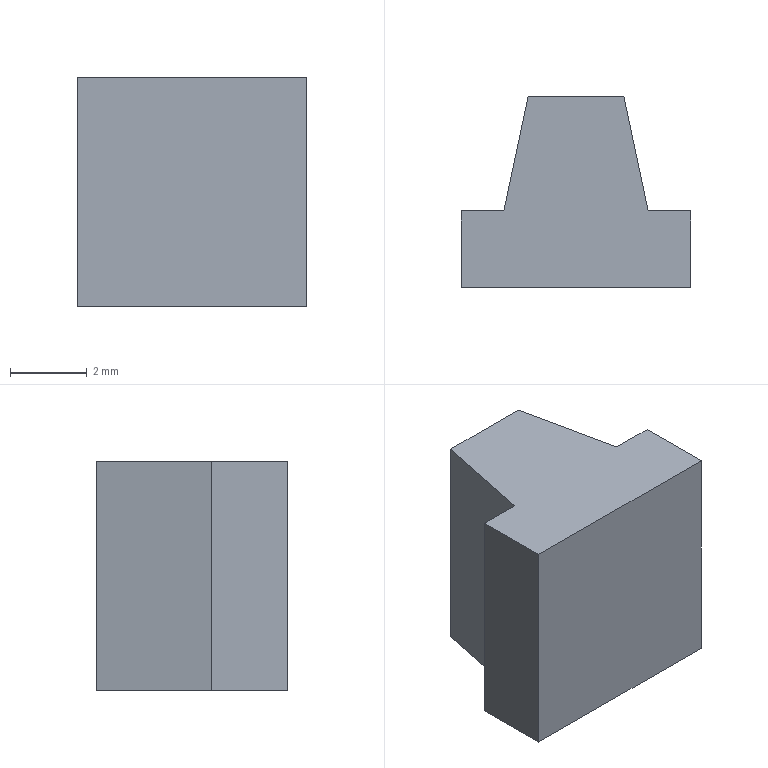Part | SolidWorks | features Extrusion 1 | 1 solid | 10 faces | box 6 x 5 x 6 mm | volume 128.419 mm3 | plane 10
STEP:
#1=CARTESIAN_POINT('',(3.,0.,0.));
#2=VERTEX_POINT('',#1);
#3=CARTESIAN_POINT('',(-3.,0.,0.));
#4=VERTEX_POINT('',#3);
#5=CARTESIAN_POINT('',(0.,0.,0.));
#6=DIRECTION('',(-1.,0.,0.));
#7=VECTOR('',#6,1000.);
#8=LINE('',#5,#7);
#9=EDGE_CURVE('',#2,#4,#8,.T.);
#10=ORIENTED_EDGE('',*,*,#9,.F.);
#11=CARTESIAN_POINT('',(3.,0.,6.));
#12=VERTEX_POINT('',#11);
#13=CARTESIAN_POINT('',(3.,0.,6.));
#14=DIRECTION('',(0.,0.,-1.));
#15=VECTOR('',#14,1000.);
#16=LINE('',#13,#15);
#17=EDGE_CURVE('',#12,#2,#16,.T.);
#18=ORIENTED_EDGE('',*,*,#17,.F.);
#19=CARTESIAN_POINT('',(-3.,0.,6.));
#20=VERTEX_POINT('',#19);
#21=CARTESIAN_POINT('',(0.,0.,6.));
#22=DIRECTION('',(-1.,0.,0.));
#23=VECTOR('',#22,1000.);
#24=LINE('',#21,#23);
#25=EDGE_CURVE('',#12,#20,#24,.T.);
#26=ORIENTED_EDGE('',*,*,#25,.T.);
#27=CARTESIAN_POINT('',(-3.,0.,6.));
#28=DIRECTION('',(0.,0.,-1.));
#29=VECTOR('',#28,1000.);
#30=LINE('',#27,#29);
#31=EDGE_CURVE('',#20,#4,#30,.T.);
#32=ORIENTED_EDGE('',*,*,#31,.T.);
#33=EDGE_LOOP('',(#10,#18,#26,#32));
#34=FACE_OUTER_BOUND('',#33,.T.);
#35=CARTESIAN_POINT('',(0.,0.,6.));
#36=DIRECTION('',(0.,-1.,0.));
#37=DIRECTION('',(0.,0.,-1.));
#38=AXIS2_PLACEMENT_3D('',#35,#36,#37);
#39=PLANE('',#38);
#40=ADVANCED_FACE('',(#34),#39,.T.);
#41=CARTESIAN_POINT('',(3.,2.,0.));
#42=VERTEX_POINT('',#41);
#43=CARTESIAN_POINT('',(3.,0.,0.));
#44=DIRECTION('',(0.,-1.,0.));
#45=VECTOR('',#44,1000.);
#46=LINE('',#43,#45);
#47=EDGE_CURVE('',#42,#2,#46,.T.);
#48=ORIENTED_EDGE('',*,*,#47,.F.);
#49=CARTESIAN_POINT('',(3.,2.,6.));
#50=VERTEX_POINT('',#49);
#51=CARTESIAN_POINT('',(3.,2.,6.));
#52=DIRECTION('',(0.,0.,-1.));
#53=VECTOR('',#52,1000.);
#54=LINE('',#51,#53);
#55=EDGE_CURVE('',#50,#42,#54,.T.);
#56=ORIENTED_EDGE('',*,*,#55,.F.);
#57=CARTESIAN_POINT('',(3.,0.,6.));
#58=DIRECTION('',(0.,-1.,0.));
#59=VECTOR('',#58,1000.);
#60=LINE('',#57,#59);
#61=EDGE_CURVE('',#50,#12,#60,.T.);
#62=ORIENTED_EDGE('',*,*,#61,.T.);
#63=ORIENTED_EDGE('',*,*,#17,.T.);
#64=EDGE_LOOP('',(#48,#56,#62,#63));
#65=FACE_OUTER_BOUND('',#64,.T.);
#66=CARTESIAN_POINT('',(3.,0.,6.));
#67=DIRECTION('',(1.,0.,0.));
#68=DIRECTION('',(0.,0.,-1.));
#69=AXIS2_PLACEMENT_3D('',#66,#67,#68);
#70=PLANE('',#69);
#71=ADVANCED_FACE('',(#65),#70,.T.);
#72=CARTESIAN_POINT('',(1.884,2.,0.));
#73=VERTEX_POINT('',#72);
#74=CARTESIAN_POINT('',(0.,2.,0.));
#75=DIRECTION('',(1.,0.,0.));
#76=VECTOR('',#75,1000.);
#77=LINE('',#74,#76);
#78=EDGE_CURVE('',#73,#42,#77,.T.);
#79=ORIENTED_EDGE('',*,*,#78,.F.);
#80=CARTESIAN_POINT('',(1.884,2.,6.));
#81=VERTEX_POINT('',#80);
#82=CARTESIAN_POINT('',(1.884,2.,6.));
#83=DIRECTION('',(0.,0.,-1.));
#84=VECTOR('',#83,1000.);
#85=LINE('',#82,#84);
#86=EDGE_CURVE('',#81,#73,#85,.T.);
#87=ORIENTED_EDGE('',*,*,#86,.F.);
#88=CARTESIAN_POINT('',(0.,2.,6.));
#89=DIRECTION('',(1.,0.,0.));
#90=VECTOR('',#89,1000.);
#91=LINE('',#88,#90);
#92=EDGE_CURVE('',#81,#50,#91,.T.);
#93=ORIENTED_EDGE('',*,*,#92,.T.);
#94=ORIENTED_EDGE('',*,*,#55,.T.);
#95=EDGE_LOOP('',(#79,#87,#93,#94));
#96=FACE_OUTER_BOUND('',#95,.T.);
#97=CARTESIAN_POINT('',(0.,2.,6.));
#98=DIRECTION('',(0.,1.,0.));
#99=DIRECTION('',(0.,0.,1.));
#100=AXIS2_PLACEMENT_3D('',#97,#98,#99);
#101=PLANE('',#100);
#102=ADVANCED_FACE('',(#96),#101,.T.);
#103=CARTESIAN_POINT('',(1.25,5.,0.));
#104=VERTEX_POINT('',#103);
#105=CARTESIAN_POINT('',(2.209,0.467,0.));
#106=DIRECTION('',(0.2069,-0.9784,0.));
#107=VECTOR('',#106,1000.);
#108=LINE('',#105,#107);
#109=EDGE_CURVE('',#104,#73,#108,.T.);
#110=ORIENTED_EDGE('',*,*,#109,.F.);
#111=CARTESIAN_POINT('',(1.25,5.,6.));
#112=VERTEX_POINT('',#111);
#113=CARTESIAN_POINT('',(1.25,5.,6.));
#114=DIRECTION('',(0.,0.,-1.));
#115=VECTOR('',#114,1000.);
#116=LINE('',#113,#115);
#117=EDGE_CURVE('',#112,#104,#116,.T.);
#118=ORIENTED_EDGE('',*,*,#117,.F.);
#119=CARTESIAN_POINT('',(2.209,0.467,6.));
#120=DIRECTION('',(0.2069,-0.9784,0.));
#121=VECTOR('',#120,1000.);
#122=LINE('',#119,#121);
#123=EDGE_CURVE('',#112,#81,#122,.T.);
#124=ORIENTED_EDGE('',*,*,#123,.T.);
#125=ORIENTED_EDGE('',*,*,#86,.T.);
#126=EDGE_LOOP('',(#110,#118,#124,#125));
#127=FACE_OUTER_BOUND('',#126,.T.);
#128=CARTESIAN_POINT('',(2.209,0.467,6.));
#129=DIRECTION('',(0.9784,0.2069,0.));
#130=DIRECTION('',(-0.2069,0.9784,0.));
#131=AXIS2_PLACEMENT_3D('',#128,#129,#130);
#132=PLANE('',#131);
#133=ADVANCED_FACE('',(#127),#132,.T.);
#134=CARTESIAN_POINT('',(-1.25,5.,0.));
#135=VERTEX_POINT('',#134);
#136=CARTESIAN_POINT('',(0.,5.,0.));
#137=DIRECTION('',(1.,0.,0.));
#138=VECTOR('',#137,1000.);
#139=LINE('',#136,#138);
#140=EDGE_CURVE('',#135,#104,#139,.T.);
#141=ORIENTED_EDGE('',*,*,#140,.F.);
#142=CARTESIAN_POINT('',(-1.25,5.,6.));
#143=VERTEX_POINT('',#142);
#144=CARTESIAN_POINT('',(-1.25,5.,6.));
#145=DIRECTION('',(0.,0.,-1.));
#146=VECTOR('',#145,1000.);
#147=LINE('',#144,#146);
#148=EDGE_CURVE('',#143,#135,#147,.T.);
#149=ORIENTED_EDGE('',*,*,#148,.F.);
#150=CARTESIAN_POINT('',(0.,5.,6.));
#151=DIRECTION('',(1.,0.,0.));
#152=VECTOR('',#151,1000.);
#153=LINE('',#150,#152);
#154=EDGE_CURVE('',#143,#112,#153,.T.);
#155=ORIENTED_EDGE('',*,*,#154,.T.);
#156=ORIENTED_EDGE('',*,*,#117,.T.);
#157=EDGE_LOOP('',(#141,#149,#155,#156));
#158=FACE_OUTER_BOUND('',#157,.T.);
#159=CARTESIAN_POINT('',(0.,5.,6.));
#160=DIRECTION('',(0.,1.,0.));
#161=DIRECTION('',(0.,0.,1.));
#162=AXIS2_PLACEMENT_3D('',#159,#160,#161);
#163=PLANE('',#162);
#164=ADVANCED_FACE('',(#158),#163,.T.);
#165=CARTESIAN_POINT('',(-1.884,2.,0.));
#166=VERTEX_POINT('',#165);
#167=CARTESIAN_POINT('',(-2.209,0.467,0.));
#168=DIRECTION('',(0.2069,0.9784,0.));
#169=VECTOR('',#168,1000.);
#170=LINE('',#167,#169);
#171=EDGE_CURVE('',#166,#135,#170,.T.);
#172=ORIENTED_EDGE('',*,*,#171,.F.);
#173=CARTESIAN_POINT('',(-1.884,2.,6.));
#174=VERTEX_POINT('',#173);
#175=CARTESIAN_POINT('',(-1.884,2.,6.));
#176=DIRECTION('',(0.,0.,-1.));
#177=VECTOR('',#176,1000.);
#178=LINE('',#175,#177);
#179=EDGE_CURVE('',#174,#166,#178,.T.);
#180=ORIENTED_EDGE('',*,*,#179,.F.);
#181=CARTESIAN_POINT('',(-2.209,0.467,6.));
#182=DIRECTION('',(0.2069,0.9784,0.));
#183=VECTOR('',#182,1000.);
#184=LINE('',#181,#183);
#185=EDGE_CURVE('',#174,#143,#184,.T.);
#186=ORIENTED_EDGE('',*,*,#185,.T.);
#187=ORIENTED_EDGE('',*,*,#148,.T.);
#188=EDGE_LOOP('',(#172,#180,#186,#187));
#189=FACE_OUTER_BOUND('',#188,.T.);
#190=CARTESIAN_POINT('',(-2.209,0.467,6.));
#191=DIRECTION('',(-0.9784,0.2069,0.));
#192=DIRECTION('',(-0.2069,-0.9784,0.));
#193=AXIS2_PLACEMENT_3D('',#190,#191,#192);
#194=PLANE('',#193);
#195=ADVANCED_FACE('',(#189),#194,.T.);
#196=CARTESIAN_POINT('',(-3.,2.,0.));
#197=VERTEX_POINT('',#196);
#198=CARTESIAN_POINT('',(0.,2.,0.));
#199=DIRECTION('',(1.,0.,0.));
#200=VECTOR('',#199,1000.);
#201=LINE('',#198,#200);
#202=EDGE_CURVE('',#197,#166,#201,.T.);
#203=ORIENTED_EDGE('',*,*,#202,.F.);
#204=CARTESIAN_POINT('',(-3.,2.,6.));
#205=VERTEX_POINT('',#204);
#206=CARTESIAN_POINT('',(-3.,2.,6.));
#207=DIRECTION('',(0.,0.,-1.));
#208=VECTOR('',#207,1000.);
#209=LINE('',#206,#208);
#210=EDGE_CURVE('',#205,#197,#209,.T.);
#211=ORIENTED_EDGE('',*,*,#210,.F.);
#212=CARTESIAN_POINT('',(0.,2.,6.));
#213=DIRECTION('',(1.,0.,0.));
#214=VECTOR('',#213,1000.);
#215=LINE('',#212,#214);
#216=EDGE_CURVE('',#205,#174,#215,.T.);
#217=ORIENTED_EDGE('',*,*,#216,.T.);
#218=ORIENTED_EDGE('',*,*,#179,.T.);
#219=EDGE_LOOP('',(#203,#211,#217,#218));
#220=FACE_OUTER_BOUND('',#219,.T.);
#221=CARTESIAN_POINT('',(0.,2.,6.));
#222=DIRECTION('',(0.,1.,0.));
#223=DIRECTION('',(0.,0.,1.));
#224=AXIS2_PLACEMENT_3D('',#221,#222,#223);
#225=PLANE('',#224);
#226=ADVANCED_FACE('',(#220),#225,.T.);
#227=CARTESIAN_POINT('',(-3.,0.,0.));
#228=DIRECTION('',(0.,1.,0.));
#229=VECTOR('',#228,1000.);
#230=LINE('',#227,#229);
#231=EDGE_CURVE('',#4,#197,#230,.T.);
#232=ORIENTED_EDGE('',*,*,#231,.F.);
#233=ORIENTED_EDGE('',*,*,#31,.F.);
#234=CARTESIAN_POINT('',(-3.,0.,6.));
#235=DIRECTION('',(0.,1.,0.));
#236=VECTOR('',#235,1000.);
#237=LINE('',#234,#236);
#238=EDGE_CURVE('',#20,#205,#237,.T.);
#239=ORIENTED_EDGE('',*,*,#238,.T.);
#240=ORIENTED_EDGE('',*,*,#210,.T.);
#241=EDGE_LOOP('',(#232,#233,#239,#240));
#242=FACE_OUTER_BOUND('',#241,.T.);
#243=CARTESIAN_POINT('',(-3.,0.,6.));
#244=DIRECTION('',(-1.,0.,0.));
#245=DIRECTION('',(0.,0.,1.));
#246=AXIS2_PLACEMENT_3D('',#243,#244,#245);
#247=PLANE('',#246);
#248=ADVANCED_FACE('',(#242),#247,.T.);
#249=ORIENTED_EDGE('',*,*,#25,.F.);
#250=ORIENTED_EDGE('',*,*,#61,.F.);
#251=ORIENTED_EDGE('',*,*,#92,.F.);
#252=ORIENTED_EDGE('',*,*,#123,.F.);
#253=ORIENTED_EDGE('',*,*,#154,.F.);
#254=ORIENTED_EDGE('',*,*,#185,.F.);
#255=ORIENTED_EDGE('',*,*,#216,.F.);
#256=ORIENTED_EDGE('',*,*,#238,.F.);
#257=EDGE_LOOP('',(#249,#250,#251,#252,#253,#254,#255,#256));
#258=FACE_OUTER_BOUND('',#257,.T.);
#259=CARTESIAN_POINT('',(0.,0.,6.));
#260=DIRECTION('',(0.,0.,1.));
#261=DIRECTION('',(1.,0.,0.));
#262=AXIS2_PLACEMENT_3D('',#259,#260,#261);
#263=PLANE('',#262);
#264=ADVANCED_FACE('',(#258),#263,.T.);
#265=ORIENTED_EDGE('',*,*,#9,.T.);
#266=ORIENTED_EDGE('',*,*,#231,.T.);
#267=ORIENTED_EDGE('',*,*,#202,.T.);
#268=ORIENTED_EDGE('',*,*,#171,.T.);
#269=ORIENTED_EDGE('',*,*,#140,.T.);
#270=ORIENTED_EDGE('',*,*,#109,.T.);
#271=ORIENTED_EDGE('',*,*,#78,.T.);
#272=ORIENTED_EDGE('',*,*,#47,.T.);
#273=EDGE_LOOP('',(#265,#266,#267,#268,#269,#270,#271,#272));
#274=FACE_OUTER_BOUND('',#273,.T.);
#275=CARTESIAN_POINT('',(0.,0.,0.));
#276=DIRECTION('',(0.,0.,1.));
#277=DIRECTION('',(1.,0.,0.));
#278=AXIS2_PLACEMENT_3D('',#275,#276,#277);
#279=PLANE('',#278);
#280=ADVANCED_FACE('',(#274),#279,.F.);
#281=CLOSED_SHELL('',(#40,#71,#102,#133,#164,#195,#226,#248,#264,#280));
#282=MANIFOLD_SOLID_BREP('',#281);
#283=CARTESIAN_POINT('',(0.,0.,0.));
#284=DIRECTION('',(0.,0.,1.));
#285=DIRECTION('',(1.,0.,0.));
#286=AXIS2_PLACEMENT_3D('',#283,#284,#285);
#287=(LENGTH_UNIT()NAMED_UNIT(*)SI_UNIT(.MILLI.,.METRE.));
#288=UNCERTAINTY_MEASURE_WITH_UNIT(LENGTH_MEASURE(0.00001),#287,'','');
#289=(NAMED_UNIT(*)PLANE_ANGLE_UNIT()SI_UNIT($,.RADIAN.));
#290=(NAMED_UNIT(*)SI_UNIT($,.STERADIAN.)SOLID_ANGLE_UNIT());
#291=(GEOMETRIC_REPRESENTATION_CONTEXT(3)GLOBAL_UNCERTAINTY_ASSIGNED_CONTEXT((#288))GLOBAL_UNIT_ASSIGNED_CONTEXT((#287,#289,#290))REPRESENTATION_CONTEXT('',''));
#292=ADVANCED_BREP_SHAPE_REPRESENTATION('',(#282,#286),#291);